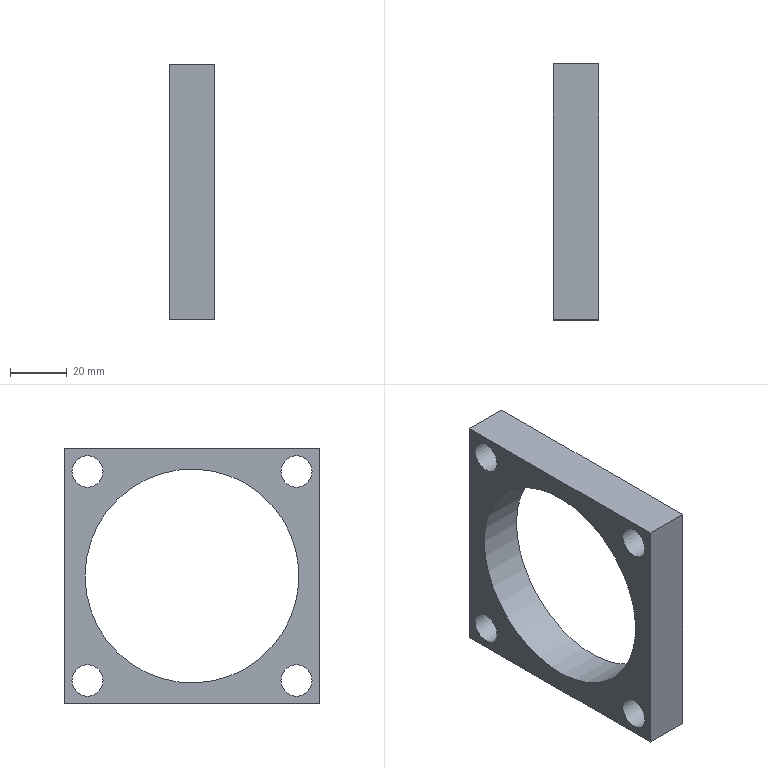Part | NX | features MAIN_BODY 2 | 1 solid | 11 faces | box 16 x 90 x 90 mm | volume 52455 mm3 | plane 6 | cylinder 5 | commonest cylinder face diameters 11 x4 75.2 x1
STEP:
#1=CARTESIAN_POINT('',(-571.,135.,-250.));
#2=VERTEX_POINT('',#1);
#3=CARTESIAN_POINT('',(-571.,135.,-340.));
#4=VERTEX_POINT('',#3);
#5=CARTESIAN_POINT('',(-571.,135.,-250.));
#6=DIRECTION('',(0.,0.,-1.));
#7=VECTOR('',#6,1000.);
#8=LINE('',#5,#7);
#9=EDGE_CURVE('',#2,#4,#8,.T.);
#10=ORIENTED_EDGE('',*,*,#9,.T.);
#11=CARTESIAN_POINT('',(-555.,135.,-340.));
#12=VERTEX_POINT('',#11);
#13=CARTESIAN_POINT('',(-555.,135.,-340.));
#14=DIRECTION('',(-1.,0.,0.));
#15=VECTOR('',#14,1000.);
#16=LINE('',#13,#15);
#17=EDGE_CURVE('',#12,#4,#16,.T.);
#18=ORIENTED_EDGE('',*,*,#17,.F.);
#19=CARTESIAN_POINT('',(-555.,135.,-250.));
#20=VERTEX_POINT('',#19);
#21=CARTESIAN_POINT('',(-555.,135.,-250.));
#22=DIRECTION('',(0.,0.,-1.));
#23=VECTOR('',#22,1000.);
#24=LINE('',#21,#23);
#25=EDGE_CURVE('',#20,#12,#24,.T.);
#26=ORIENTED_EDGE('',*,*,#25,.F.);
#27=CARTESIAN_POINT('',(-555.,135.,-250.));
#28=DIRECTION('',(-1.,0.,0.));
#29=VECTOR('',#28,1000.);
#30=LINE('',#27,#29);
#31=EDGE_CURVE('',#20,#2,#30,.T.);
#32=ORIENTED_EDGE('',*,*,#31,.T.);
#33=EDGE_LOOP('',(#10,#18,#26,#32));
#34=FACE_BOUND('',#33,.T.);
#35=CARTESIAN_POINT('',(-555.,135.,-250.));
#36=DIRECTION('',(0.,1.,0.));
#37=DIRECTION('',(0.,0.,-1.));
#38=AXIS2_PLACEMENT_3D('',#35,#36,#37);
#39=PLANE('',#38);
#40=ADVANCED_FACE('',(#34),#39,.F.);
#41=CARTESIAN_POINT('',(-571.,225.,-340.));
#42=VERTEX_POINT('',#41);
#43=CARTESIAN_POINT('',(-571.,135.,-340.));
#44=DIRECTION('',(0.,1.,0.));
#45=VECTOR('',#44,1000.);
#46=LINE('',#43,#45);
#47=EDGE_CURVE('',#4,#42,#46,.T.);
#48=ORIENTED_EDGE('',*,*,#47,.T.);
#49=CARTESIAN_POINT('',(-555.,225.,-340.));
#50=VERTEX_POINT('',#49);
#51=CARTESIAN_POINT('',(-555.,225.,-340.));
#52=DIRECTION('',(-1.,0.,0.));
#53=VECTOR('',#52,1000.);
#54=LINE('',#51,#53);
#55=EDGE_CURVE('',#50,#42,#54,.T.);
#56=ORIENTED_EDGE('',*,*,#55,.F.);
#57=CARTESIAN_POINT('',(-555.,135.,-340.));
#58=DIRECTION('',(0.,1.,0.));
#59=VECTOR('',#58,1000.);
#60=LINE('',#57,#59);
#61=EDGE_CURVE('',#12,#50,#60,.T.);
#62=ORIENTED_EDGE('',*,*,#61,.F.);
#63=ORIENTED_EDGE('',*,*,#17,.T.);
#64=EDGE_LOOP('',(#48,#56,#62,#63));
#65=FACE_BOUND('',#64,.T.);
#66=CARTESIAN_POINT('',(-555.,135.,-340.));
#67=DIRECTION('',(0.,0.,1.));
#68=DIRECTION('',(0.,1.,0.));
#69=AXIS2_PLACEMENT_3D('',#66,#67,#68);
#70=PLANE('',#69);
#71=ADVANCED_FACE('',(#65),#70,.F.);
#72=CARTESIAN_POINT('',(-571.,225.,-250.));
#73=VERTEX_POINT('',#72);
#74=CARTESIAN_POINT('',(-571.,225.,-340.));
#75=DIRECTION('',(0.,0.,1.));
#76=VECTOR('',#75,1000.);
#77=LINE('',#74,#76);
#78=EDGE_CURVE('',#42,#73,#77,.T.);
#79=ORIENTED_EDGE('',*,*,#78,.T.);
#80=CARTESIAN_POINT('',(-555.,225.,-250.));
#81=VERTEX_POINT('',#80);
#82=CARTESIAN_POINT('',(-555.,225.,-250.));
#83=DIRECTION('',(-1.,0.,0.));
#84=VECTOR('',#83,1000.);
#85=LINE('',#82,#84);
#86=EDGE_CURVE('',#81,#73,#85,.T.);
#87=ORIENTED_EDGE('',*,*,#86,.F.);
#88=CARTESIAN_POINT('',(-555.,225.,-340.));
#89=DIRECTION('',(0.,0.,1.));
#90=VECTOR('',#89,1000.);
#91=LINE('',#88,#90);
#92=EDGE_CURVE('',#50,#81,#91,.T.);
#93=ORIENTED_EDGE('',*,*,#92,.F.);
#94=ORIENTED_EDGE('',*,*,#55,.T.);
#95=EDGE_LOOP('',(#79,#87,#93,#94));
#96=FACE_BOUND('',#95,.T.);
#97=CARTESIAN_POINT('',(-555.,225.,-340.));
#98=DIRECTION('',(0.,-1.,0.));
#99=DIRECTION('',(1.,0.,0.));
#100=AXIS2_PLACEMENT_3D('',#97,#98,#99);
#101=PLANE('',#100);
#102=ADVANCED_FACE('',(#96),#101,.F.);
#103=CARTESIAN_POINT('',(-571.,225.,-250.));
#104=DIRECTION('',(0.,-1.,0.));
#105=VECTOR('',#104,1000.);
#106=LINE('',#103,#105);
#107=EDGE_CURVE('',#73,#2,#106,.T.);
#108=ORIENTED_EDGE('',*,*,#107,.T.);
#109=ORIENTED_EDGE('',*,*,#31,.F.);
#110=CARTESIAN_POINT('',(-555.,225.,-250.));
#111=DIRECTION('',(0.,-1.,0.));
#112=VECTOR('',#111,1000.);
#113=LINE('',#110,#112);
#114=EDGE_CURVE('',#81,#20,#113,.T.);
#115=ORIENTED_EDGE('',*,*,#114,.F.);
#116=ORIENTED_EDGE('',*,*,#86,.T.);
#117=EDGE_LOOP('',(#108,#109,#115,#116));
#118=FACE_BOUND('',#117,.T.);
#119=CARTESIAN_POINT('',(-555.,225.,-250.));
#120=DIRECTION('',(0.,0.,-1.));
#121=DIRECTION('',(1.,0.,0.));
#122=AXIS2_PLACEMENT_3D('',#119,#120,#121);
#123=PLANE('',#122);
#124=ADVANCED_FACE('',(#118),#123,.F.);
#125=CARTESIAN_POINT('',(-555.,217.6,-295.));
#126=VERTEX_POINT('',#125);
#127=CARTESIAN_POINT('',(-555.,180.,-295.));
#128=DIRECTION('',(1.,0.,0.));
#129=DIRECTION('',(0.,1.,0.));
#130=AXIS2_PLACEMENT_3D('',#127,#128,#129);
#131=CIRCLE('',#130,37.6);
#132=EDGE_CURVE('',#126,#126,#131,.F.);
#133=ORIENTED_EDGE('',*,*,#132,.F.);
#134=EDGE_LOOP('',(#133));
#135=FACE_BOUND('',#134,.T.);
#136=CARTESIAN_POINT('',(-571.,217.6,-295.));
#137=VERTEX_POINT('',#136);
#138=CARTESIAN_POINT('',(-571.,180.,-295.));
#139=DIRECTION('',(1.,0.,0.));
#140=DIRECTION('',(0.,1.,0.));
#141=AXIS2_PLACEMENT_3D('',#138,#139,#140);
#142=CIRCLE('',#141,37.6);
#143=EDGE_CURVE('',#137,#137,#142,.F.);
#144=ORIENTED_EDGE('',*,*,#143,.T.);
#145=EDGE_LOOP('',(#144));
#146=FACE_BOUND('',#145,.T.);
#147=CARTESIAN_POINT('',(-555.,180.,-295.));
#148=DIRECTION('',(-1.,0.,0.));
#149=DIRECTION('',(0.,-1.,0.));
#150=AXIS2_PLACEMENT_3D('',#147,#148,#149);
#151=CYLINDRICAL_SURFACE('',#150,37.6);
#152=ADVANCED_FACE('',(#135,#146),#151,.F.);
#153=CARTESIAN_POINT('',(-555.,222.25,-331.75));
#154=VERTEX_POINT('',#153);
#155=CARTESIAN_POINT('',(-555.,216.75,-331.75));
#156=DIRECTION('',(1.,0.,0.));
#157=DIRECTION('',(0.,1.,0.));
#158=AXIS2_PLACEMENT_3D('',#155,#156,#157);
#159=CIRCLE('',#158,5.5);
#160=EDGE_CURVE('',#154,#154,#159,.T.);
#161=ORIENTED_EDGE('',*,*,#160,.F.);
#162=EDGE_LOOP('',(#161));
#163=FACE_BOUND('',#162,.T.);
#164=CARTESIAN_POINT('',(-555.,148.75,-331.75));
#165=VERTEX_POINT('',#164);
#166=CARTESIAN_POINT('',(-555.,143.25,-331.75));
#167=DIRECTION('',(1.,0.,0.));
#168=DIRECTION('',(0.,1.,0.));
#169=AXIS2_PLACEMENT_3D('',#166,#167,#168);
#170=CIRCLE('',#169,5.5);
#171=EDGE_CURVE('',#165,#165,#170,.T.);
#172=ORIENTED_EDGE('',*,*,#171,.F.);
#173=EDGE_LOOP('',(#172));
#174=FACE_BOUND('',#173,.T.);
#175=CARTESIAN_POINT('',(-555.,148.75,-258.25));
#176=VERTEX_POINT('',#175);
#177=CARTESIAN_POINT('',(-555.,143.25,-258.25));
#178=DIRECTION('',(1.,0.,0.));
#179=DIRECTION('',(0.,1.,0.));
#180=AXIS2_PLACEMENT_3D('',#177,#178,#179);
#181=CIRCLE('',#180,5.5);
#182=EDGE_CURVE('',#176,#176,#181,.T.);
#183=ORIENTED_EDGE('',*,*,#182,.F.);
#184=EDGE_LOOP('',(#183));
#185=FACE_BOUND('',#184,.T.);
#186=CARTESIAN_POINT('',(-555.,222.25,-258.25));
#187=VERTEX_POINT('',#186);
#188=CARTESIAN_POINT('',(-555.,216.75,-258.25));
#189=DIRECTION('',(1.,0.,0.));
#190=DIRECTION('',(0.,1.,0.));
#191=AXIS2_PLACEMENT_3D('',#188,#189,#190);
#192=CIRCLE('',#191,5.5);
#193=EDGE_CURVE('',#187,#187,#192,.T.);
#194=ORIENTED_EDGE('',*,*,#193,.F.);
#195=EDGE_LOOP('',(#194));
#196=FACE_BOUND('',#195,.T.);
#197=ORIENTED_EDGE('',*,*,#25,.T.);
#198=ORIENTED_EDGE('',*,*,#61,.T.);
#199=ORIENTED_EDGE('',*,*,#92,.T.);
#200=ORIENTED_EDGE('',*,*,#114,.T.);
#201=EDGE_LOOP('',(#197,#198,#199,#200));
#202=FACE_BOUND('',#201,.T.);
#203=ORIENTED_EDGE('',*,*,#132,.T.);
#204=EDGE_LOOP('',(#203));
#205=FACE_BOUND('',#204,.T.);
#206=CARTESIAN_POINT('',(-555.,135.,-340.));
#207=DIRECTION('',(1.,0.,0.));
#208=DIRECTION('',(0.,1.,0.));
#209=AXIS2_PLACEMENT_3D('',#206,#207,#208);
#210=PLANE('',#209);
#211=ADVANCED_FACE('',(#163,#174,#185,#196,#202,#205),#210,.T.);
#212=CARTESIAN_POINT('',(-571.,222.25,-331.75));
#213=VERTEX_POINT('',#212);
#214=CARTESIAN_POINT('',(-571.,216.75,-331.75));
#215=DIRECTION('',(1.,0.,0.));
#216=DIRECTION('',(0.,1.,0.));
#217=AXIS2_PLACEMENT_3D('',#214,#215,#216);
#218=CIRCLE('',#217,5.5);
#219=EDGE_CURVE('',#213,#213,#218,.T.);
#220=ORIENTED_EDGE('',*,*,#219,.T.);
#221=EDGE_LOOP('',(#220));
#222=FACE_BOUND('',#221,.T.);
#223=CARTESIAN_POINT('',(-571.,148.75,-331.75));
#224=VERTEX_POINT('',#223);
#225=CARTESIAN_POINT('',(-571.,143.25,-331.75));
#226=DIRECTION('',(1.,0.,0.));
#227=DIRECTION('',(0.,1.,0.));
#228=AXIS2_PLACEMENT_3D('',#225,#226,#227);
#229=CIRCLE('',#228,5.5);
#230=EDGE_CURVE('',#224,#224,#229,.T.);
#231=ORIENTED_EDGE('',*,*,#230,.T.);
#232=EDGE_LOOP('',(#231));
#233=FACE_BOUND('',#232,.T.);
#234=CARTESIAN_POINT('',(-571.,148.75,-258.25));
#235=VERTEX_POINT('',#234);
#236=CARTESIAN_POINT('',(-571.,143.25,-258.25));
#237=DIRECTION('',(1.,0.,0.));
#238=DIRECTION('',(0.,1.,0.));
#239=AXIS2_PLACEMENT_3D('',#236,#237,#238);
#240=CIRCLE('',#239,5.5);
#241=EDGE_CURVE('',#235,#235,#240,.T.);
#242=ORIENTED_EDGE('',*,*,#241,.T.);
#243=EDGE_LOOP('',(#242));
#244=FACE_BOUND('',#243,.T.);
#245=CARTESIAN_POINT('',(-571.,222.25,-258.25));
#246=VERTEX_POINT('',#245);
#247=CARTESIAN_POINT('',(-571.,216.75,-258.25));
#248=DIRECTION('',(1.,0.,0.));
#249=DIRECTION('',(0.,1.,0.));
#250=AXIS2_PLACEMENT_3D('',#247,#248,#249);
#251=CIRCLE('',#250,5.5);
#252=EDGE_CURVE('',#246,#246,#251,.T.);
#253=ORIENTED_EDGE('',*,*,#252,.T.);
#254=EDGE_LOOP('',(#253));
#255=FACE_BOUND('',#254,.T.);
#256=ORIENTED_EDGE('',*,*,#9,.F.);
#257=ORIENTED_EDGE('',*,*,#107,.F.);
#258=ORIENTED_EDGE('',*,*,#78,.F.);
#259=ORIENTED_EDGE('',*,*,#47,.F.);
#260=EDGE_LOOP('',(#256,#257,#258,#259));
#261=FACE_BOUND('',#260,.T.);
#262=ORIENTED_EDGE('',*,*,#143,.F.);
#263=EDGE_LOOP('',(#262));
#264=FACE_BOUND('',#263,.T.);
#265=CARTESIAN_POINT('',(-571.,135.,-340.));
#266=DIRECTION('',(1.,0.,0.));
#267=DIRECTION('',(0.,1.,0.));
#268=AXIS2_PLACEMENT_3D('',#265,#266,#267);
#269=PLANE('',#268);
#270=ADVANCED_FACE('',(#222,#233,#244,#255,#261,#264),#269,.F.);
#271=ORIENTED_EDGE('',*,*,#193,.T.);
#272=EDGE_LOOP('',(#271));
#273=FACE_BOUND('',#272,.T.);
#274=ORIENTED_EDGE('',*,*,#252,.F.);
#275=EDGE_LOOP('',(#274));
#276=FACE_BOUND('',#275,.T.);
#277=CARTESIAN_POINT('',(-394.,216.75,-258.25));
#278=DIRECTION('',(-1.,0.,0.));
#279=DIRECTION('',(0.,-1.,0.));
#280=AXIS2_PLACEMENT_3D('',#277,#278,#279);
#281=CYLINDRICAL_SURFACE('',#280,5.5);
#282=ADVANCED_FACE('',(#273,#276),#281,.F.);
#283=ORIENTED_EDGE('',*,*,#182,.T.);
#284=EDGE_LOOP('',(#283));
#285=FACE_BOUND('',#284,.T.);
#286=ORIENTED_EDGE('',*,*,#241,.F.);
#287=EDGE_LOOP('',(#286));
#288=FACE_BOUND('',#287,.T.);
#289=CARTESIAN_POINT('',(-394.,143.25,-258.25));
#290=DIRECTION('',(-1.,0.,0.));
#291=DIRECTION('',(0.,-1.,0.));
#292=AXIS2_PLACEMENT_3D('',#289,#290,#291);
#293=CYLINDRICAL_SURFACE('',#292,5.5);
#294=ADVANCED_FACE('',(#285,#288),#293,.F.);
#295=ORIENTED_EDGE('',*,*,#171,.T.);
#296=EDGE_LOOP('',(#295));
#297=FACE_BOUND('',#296,.T.);
#298=ORIENTED_EDGE('',*,*,#230,.F.);
#299=EDGE_LOOP('',(#298));
#300=FACE_BOUND('',#299,.T.);
#301=CARTESIAN_POINT('',(-394.,143.25,-331.75));
#302=DIRECTION('',(-1.,0.,0.));
#303=DIRECTION('',(0.,-1.,0.));
#304=AXIS2_PLACEMENT_3D('',#301,#302,#303);
#305=CYLINDRICAL_SURFACE('',#304,5.5);
#306=ADVANCED_FACE('',(#297,#300),#305,.F.);
#307=ORIENTED_EDGE('',*,*,#160,.T.);
#308=EDGE_LOOP('',(#307));
#309=FACE_BOUND('',#308,.T.);
#310=ORIENTED_EDGE('',*,*,#219,.F.);
#311=EDGE_LOOP('',(#310));
#312=FACE_BOUND('',#311,.T.);
#313=CARTESIAN_POINT('',(-394.,216.75,-331.75));
#314=DIRECTION('',(-1.,0.,0.));
#315=DIRECTION('',(0.,-1.,0.));
#316=AXIS2_PLACEMENT_3D('',#313,#314,#315);
#317=CYLINDRICAL_SURFACE('',#316,5.5);
#318=ADVANCED_FACE('',(#309,#312),#317,.F.);
#319=CLOSED_SHELL('',(#40,#71,#102,#124,#152,#211,#270,#282,#294,#306,#318));
#320=MANIFOLD_SOLID_BREP('',#319);
#321=(LENGTH_UNIT()NAMED_UNIT(*)SI_UNIT(.MILLI.,.METRE.));
#322=UNCERTAINTY_MEASURE_WITH_UNIT(LENGTH_MEASURE(0.00001),#321,'','');
#323=(NAMED_UNIT(*)PLANE_ANGLE_UNIT()SI_UNIT($,.RADIAN.));
#324=(NAMED_UNIT(*)SI_UNIT($,.STERADIAN.)SOLID_ANGLE_UNIT());
#325=(GEOMETRIC_REPRESENTATION_CONTEXT(3)GLOBAL_UNCERTAINTY_ASSIGNED_CONTEXT((#322))GLOBAL_UNIT_ASSIGNED_CONTEXT((#321,#323,#324))REPRESENTATION_CONTEXT('',''));
#326=ADVANCED_BREP_SHAPE_REPRESENTATION('',(#320),#325);